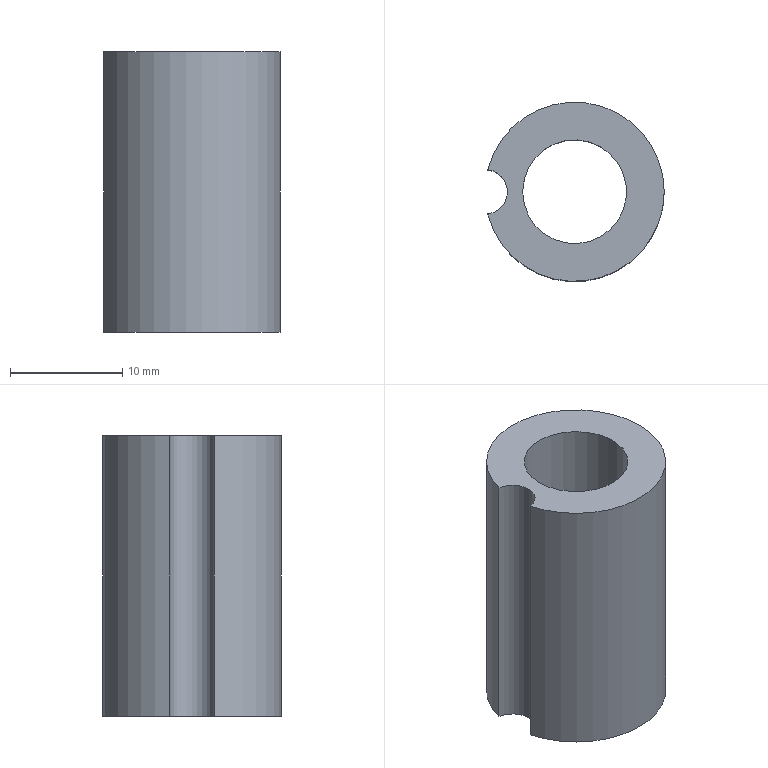Part | NX | features solid 2 | 1 solid | 7 faces | box 15.75 x 16 x 25 mm | volume 2839 mm3 | cylinder 4 | plane 3 | commonest cylinder face diameters 4 x1 9.26 x1 10.6 x1 16 x1
STEP:
#1=CARTESIAN_POINT('',(-120.262,-350.396,-62.));
#2=VERTEX_POINT('',#1);
#3=CARTESIAN_POINT('',(-120.262,-354.365,-62.));
#4=VERTEX_POINT('',#3);
#5=CARTESIAN_POINT('',(-120.512,-352.381,-62.));
#6=DIRECTION('',(0.,0.,-1.));
#7=DIRECTION('',(-1.,0.,0.));
#8=AXIS2_PLACEMENT_3D('',#5,#6,#7);
#9=CIRCLE('',#8,2.);
#10=EDGE_CURVE('',#2,#4,#9,.T.);
#11=ORIENTED_EDGE('',*,*,#10,.F.);
#12=CARTESIAN_POINT('',(-120.262,-350.396,-87.));
#13=VERTEX_POINT('',#12);
#14=CARTESIAN_POINT('',(-120.262,-350.396,-87.));
#15=DIRECTION('',(0.,0.,1.));
#16=VECTOR('',#15,1000.);
#17=LINE('',#14,#16);
#18=EDGE_CURVE('',#13,#2,#17,.T.);
#19=ORIENTED_EDGE('',*,*,#18,.F.);
#20=CARTESIAN_POINT('',(-120.262,-354.365,-87.));
#21=VERTEX_POINT('',#20);
#22=CARTESIAN_POINT('',(-120.512,-352.381,-87.));
#23=DIRECTION('',(0.,0.,-1.));
#24=DIRECTION('',(-1.,0.,0.));
#25=AXIS2_PLACEMENT_3D('',#22,#23,#24);
#26=CIRCLE('',#25,2.);
#27=EDGE_CURVE('',#13,#21,#26,.T.);
#28=ORIENTED_EDGE('',*,*,#27,.T.);
#29=CARTESIAN_POINT('',(-120.262,-354.365,-87.));
#30=DIRECTION('',(0.,0.,1.));
#31=VECTOR('',#30,1000.);
#32=LINE('',#29,#31);
#33=EDGE_CURVE('',#4,#21,#32,.F.);
#34=ORIENTED_EDGE('',*,*,#33,.F.);
#35=EDGE_LOOP('',(#11,#19,#28,#34));
#36=FACE_BOUND('',#35,.T.);
#37=CARTESIAN_POINT('',(-120.512,-352.381,-87.));
#38=DIRECTION('',(0.,0.,1.));
#39=DIRECTION('',(-1.,0.,0.));
#40=AXIS2_PLACEMENT_3D('',#37,#38,#39);
#41=CYLINDRICAL_SURFACE('',#40,2.);
#42=ADVANCED_FACE('',(#36),#41,.F.);
#43=CARTESIAN_POINT('',(-112.512,-352.381,-62.));
#44=DIRECTION('',(0.,0.,-1.));
#45=DIRECTION('',(-1.,0.,0.));
#46=AXIS2_PLACEMENT_3D('',#43,#44,#45);
#47=CIRCLE('',#46,8.);
#48=EDGE_CURVE('',#2,#4,#47,.T.);
#49=ORIENTED_EDGE('',*,*,#48,.T.);
#50=ORIENTED_EDGE('',*,*,#33,.T.);
#51=CARTESIAN_POINT('',(-112.512,-352.381,-87.));
#52=DIRECTION('',(0.,0.,-1.));
#53=DIRECTION('',(-1.,0.,0.));
#54=AXIS2_PLACEMENT_3D('',#51,#52,#53);
#55=CIRCLE('',#54,8.);
#56=EDGE_CURVE('',#13,#21,#55,.T.);
#57=ORIENTED_EDGE('',*,*,#56,.F.);
#58=ORIENTED_EDGE('',*,*,#18,.T.);
#59=EDGE_LOOP('',(#49,#50,#57,#58));
#60=FACE_BOUND('',#59,.T.);
#61=CARTESIAN_POINT('',(-112.512,-352.381,-87.));
#62=DIRECTION('',(0.,0.,1.));
#63=DIRECTION('',(-1.,0.,0.));
#64=AXIS2_PLACEMENT_3D('',#61,#62,#63);
#65=CYLINDRICAL_SURFACE('',#64,8.);
#66=ADVANCED_FACE('',(#60),#65,.T.);
#67=CARTESIAN_POINT('',(-117.812,-352.381,-87.));
#68=VERTEX_POINT('',#67);
#69=CARTESIAN_POINT('',(-112.512,-352.381,-87.));
#70=DIRECTION('',(0.,0.,-1.));
#71=DIRECTION('',(-1.,0.,0.));
#72=AXIS2_PLACEMENT_3D('',#69,#70,#71);
#73=CIRCLE('',#72,5.3);
#74=EDGE_CURVE('',#68,#68,#73,.T.);
#75=ORIENTED_EDGE('',*,*,#74,.F.);
#76=EDGE_LOOP('',(#75));
#77=FACE_BOUND('',#76,.T.);
#78=ORIENTED_EDGE('',*,*,#27,.F.);
#79=ORIENTED_EDGE('',*,*,#56,.T.);
#80=EDGE_LOOP('',(#78,#79));
#81=FACE_BOUND('',#80,.T.);
#82=CARTESIAN_POINT('',(-121.512,-352.381,-87.));
#83=DIRECTION('',(0.,0.,1.));
#84=DIRECTION('',(-1.,0.,0.));
#85=AXIS2_PLACEMENT_3D('',#82,#83,#84);
#86=PLANE('',#85);
#87=ADVANCED_FACE('',(#77,#81),#86,.F.);
#88=CARTESIAN_POINT('',(-117.142,-352.381,-62.));
#89=VERTEX_POINT('',#88);
#90=CARTESIAN_POINT('',(-112.512,-352.381,-62.));
#91=DIRECTION('',(0.,0.,-1.));
#92=DIRECTION('',(-1.,0.,0.));
#93=AXIS2_PLACEMENT_3D('',#90,#91,#92);
#94=CIRCLE('',#93,4.63);
#95=EDGE_CURVE('',#89,#89,#94,.T.);
#96=ORIENTED_EDGE('',*,*,#95,.T.);
#97=EDGE_LOOP('',(#96));
#98=FACE_BOUND('',#97,.T.);
#99=ORIENTED_EDGE('',*,*,#10,.T.);
#100=ORIENTED_EDGE('',*,*,#48,.F.);
#101=EDGE_LOOP('',(#99,#100));
#102=FACE_BOUND('',#101,.T.);
#103=CARTESIAN_POINT('',(-121.512,-352.381,-62.));
#104=DIRECTION('',(0.,0.,1.));
#105=DIRECTION('',(-1.,0.,0.));
#106=AXIS2_PLACEMENT_3D('',#103,#104,#105);
#107=PLANE('',#106);
#108=ADVANCED_FACE('',(#98,#102),#107,.T.);
#109=CARTESIAN_POINT('',(-117.142,-352.381,-70.));
#110=VERTEX_POINT('',#109);
#111=CARTESIAN_POINT('',(-112.512,-352.381,-70.));
#112=DIRECTION('',(0.,0.,-1.));
#113=DIRECTION('',(-1.,0.,0.));
#114=AXIS2_PLACEMENT_3D('',#111,#112,#113);
#115=CIRCLE('',#114,4.63);
#116=EDGE_CURVE('',#110,#110,#115,.F.);
#117=ORIENTED_EDGE('',*,*,#116,.F.);
#118=EDGE_LOOP('',(#117));
#119=FACE_BOUND('',#118,.T.);
#120=ORIENTED_EDGE('',*,*,#95,.F.);
#121=EDGE_LOOP('',(#120));
#122=FACE_BOUND('',#121,.T.);
#123=CARTESIAN_POINT('',(-112.512,-352.381,-70.));
#124=DIRECTION('',(0.,0.,1.));
#125=DIRECTION('',(-1.,0.,0.));
#126=AXIS2_PLACEMENT_3D('',#123,#124,#125);
#127=CYLINDRICAL_SURFACE('',#126,4.63);
#128=ADVANCED_FACE('',(#119,#122),#127,.F.);
#129=CARTESIAN_POINT('',(-117.812,-352.381,-70.));
#130=VERTEX_POINT('',#129);
#131=CARTESIAN_POINT('',(-112.512,-352.381,-70.));
#132=DIRECTION('',(0.,0.,-1.));
#133=DIRECTION('',(-1.,0.,0.));
#134=AXIS2_PLACEMENT_3D('',#131,#132,#133);
#135=CIRCLE('',#134,5.3);
#136=EDGE_CURVE('',#130,#130,#135,.T.);
#137=ORIENTED_EDGE('',*,*,#136,.T.);
#138=EDGE_LOOP('',(#137));
#139=FACE_BOUND('',#138,.T.);
#140=ORIENTED_EDGE('',*,*,#116,.T.);
#141=EDGE_LOOP('',(#140));
#142=FACE_BOUND('',#141,.T.);
#143=CARTESIAN_POINT('',(-112.512,-352.381,-70.));
#144=DIRECTION('',(0.,0.,1.));
#145=DIRECTION('',(-1.,0.,0.));
#146=AXIS2_PLACEMENT_3D('',#143,#144,#145);
#147=PLANE('',#146);
#148=ADVANCED_FACE('',(#139,#142),#147,.F.);
#149=ORIENTED_EDGE('',*,*,#74,.T.);
#150=EDGE_LOOP('',(#149));
#151=FACE_BOUND('',#150,.T.);
#152=ORIENTED_EDGE('',*,*,#136,.F.);
#153=EDGE_LOOP('',(#152));
#154=FACE_BOUND('',#153,.T.);
#155=CARTESIAN_POINT('',(-112.512,-352.381,-87.));
#156=DIRECTION('',(0.,0.,1.));
#157=DIRECTION('',(-1.,0.,0.));
#158=AXIS2_PLACEMENT_3D('',#155,#156,#157);
#159=CYLINDRICAL_SURFACE('',#158,5.3);
#160=ADVANCED_FACE('',(#151,#154),#159,.F.);
#161=CLOSED_SHELL('',(#42,#66,#87,#108,#128,#148,#160));
#162=MANIFOLD_SOLID_BREP('',#161);
#163=(LENGTH_UNIT()NAMED_UNIT(*)SI_UNIT(.MILLI.,.METRE.));
#164=UNCERTAINTY_MEASURE_WITH_UNIT(LENGTH_MEASURE(0.00001),#163,'','');
#165=(NAMED_UNIT(*)PLANE_ANGLE_UNIT()SI_UNIT($,.RADIAN.));
#166=(NAMED_UNIT(*)SI_UNIT($,.STERADIAN.)SOLID_ANGLE_UNIT());
#167=(GEOMETRIC_REPRESENTATION_CONTEXT(3)GLOBAL_UNCERTAINTY_ASSIGNED_CONTEXT((#164))GLOBAL_UNIT_ASSIGNED_CONTEXT((#163,#165,#166))REPRESENTATION_CONTEXT('',''));
#168=ADVANCED_BREP_SHAPE_REPRESENTATION('',(#162),#167);